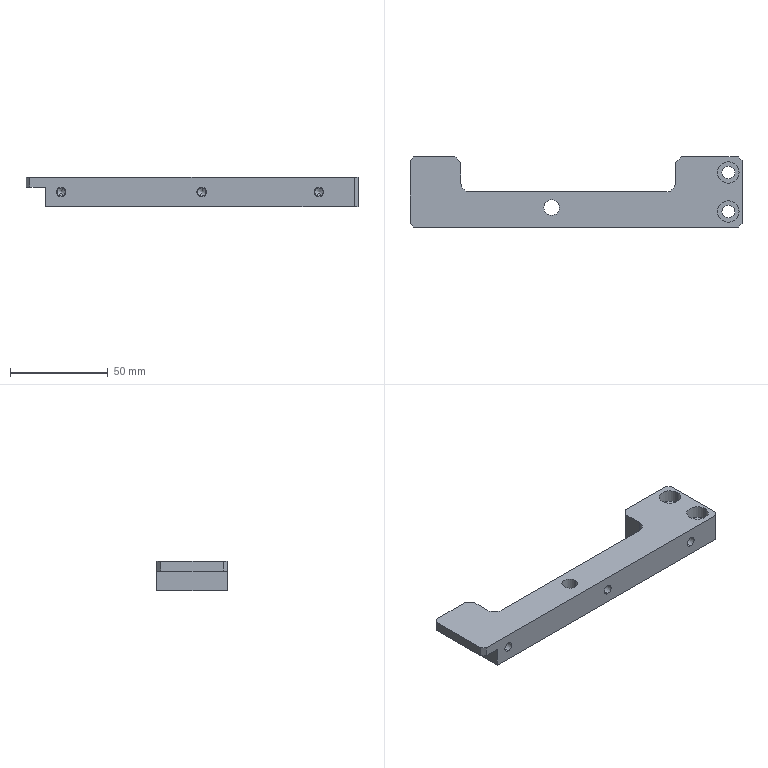Part | STEP file | J454-EBZ05-14-00-Part-1-4 | 1 solid | 53 faces | box 170 x 36 x 15 mm | volume 55026 mm3 | cylinder 24 | plane 23 | cone 6 | commonest cylinder face diameters 4.2 x6 5 x6 6.6 x4 11 x4 8 x2 10 x2